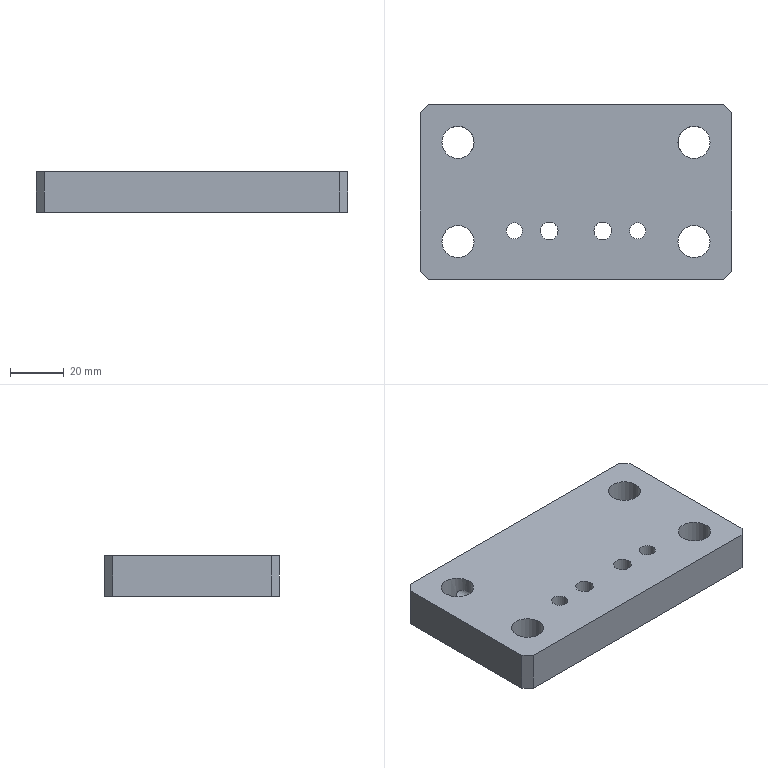Part | NX | features BREP 1 | 1 solid | 29 faces | box 116 x 65 x 15 mm | volume 102539 mm3 | cylinder 14 | plane 12 | cone 3 | commonest cylinder face diameters 5 x4 12 x4 6 x2 6.6 x2 11 x2
STEP:
#1=CARTESIAN_POINT('',(58.,0.,5.));
#2=VERTEX_POINT('',#1);
#3=CARTESIAN_POINT('',(58.,0.,7.5));
#4=DIRECTION('',(1.,0.,0.));
#5=DIRECTION('',(0.,0.,-1.));
#6=AXIS2_PLACEMENT_3D('',#3,#4,#5);
#7=CIRCLE('',#6,2.5);
#8=EDGE_CURVE('',#2,#2,#7,.T.);
#9=ORIENTED_EDGE('',*,*,#8,.F.);
#10=EDGE_LOOP('',(#9));
#11=FACE_BOUND('',#10,.T.);
#12=CARTESIAN_POINT('',(58.,-29.5,15.));
#13=VERTEX_POINT('',#12);
#14=CARTESIAN_POINT('',(58.,29.5,15.));
#15=VERTEX_POINT('',#14);
#16=CARTESIAN_POINT('',(58.,32.5,15.));
#17=DIRECTION('',(0.,1.,0.));
#18=VECTOR('',#17,1000.);
#19=LINE('',#16,#18);
#20=EDGE_CURVE('',#13,#15,#19,.T.);
#21=ORIENTED_EDGE('',*,*,#20,.F.);
#22=CARTESIAN_POINT('',(58.,-29.5,0.));
#23=VERTEX_POINT('',#22);
#24=CARTESIAN_POINT('',(58.,-29.5,15.));
#25=DIRECTION('',(0.,0.,-1.));
#26=VECTOR('',#25,1000.);
#27=LINE('',#24,#26);
#28=EDGE_CURVE('',#13,#23,#27,.T.);
#29=ORIENTED_EDGE('',*,*,#28,.T.);
#30=CARTESIAN_POINT('',(58.,29.5,0.));
#31=VERTEX_POINT('',#30);
#32=CARTESIAN_POINT('',(58.,32.5,0.));
#33=DIRECTION('',(0.,1.,0.));
#34=VECTOR('',#33,1000.);
#35=LINE('',#32,#34);
#36=EDGE_CURVE('',#23,#31,#35,.T.);
#37=ORIENTED_EDGE('',*,*,#36,.T.);
#38=CARTESIAN_POINT('',(58.,29.5,15.));
#39=DIRECTION('',(0.,0.,1.));
#40=VECTOR('',#39,1000.);
#41=LINE('',#38,#40);
#42=EDGE_CURVE('',#31,#15,#41,.T.);
#43=ORIENTED_EDGE('',*,*,#42,.T.);
#44=EDGE_LOOP('',(#21,#29,#37,#43));
#45=FACE_BOUND('',#44,.T.);
#46=CARTESIAN_POINT('',(58.,32.5,15.));
#47=DIRECTION('',(-1.,0.,0.));
#48=DIRECTION('',(0.,0.,-1.));
#49=AXIS2_PLACEMENT_3D('',#46,#47,#48);
#50=PLANE('',#49);
#51=ADVANCED_FACE('',(#11,#45),#50,.F.);
#52=CARTESIAN_POINT('',(37.5,32.5,10.));
#53=VERTEX_POINT('',#52);
#54=CARTESIAN_POINT('',(37.5,32.5,7.5));
#55=DIRECTION('',(0.,1.,0.));
#56=DIRECTION('',(0.,0.,1.));
#57=AXIS2_PLACEMENT_3D('',#54,#55,#56);
#58=CIRCLE('',#57,2.5);
#59=EDGE_CURVE('',#53,#53,#58,.T.);
#60=ORIENTED_EDGE('',*,*,#59,.F.);
#61=EDGE_LOOP('',(#60));
#62=FACE_BOUND('',#61,.T.);
#63=CARTESIAN_POINT('',(-37.5,32.5,10.));
#64=VERTEX_POINT('',#63);
#65=CARTESIAN_POINT('',(-37.5,32.5,7.5));
#66=DIRECTION('',(0.,1.,0.));
#67=DIRECTION('',(0.,0.,1.));
#68=AXIS2_PLACEMENT_3D('',#65,#66,#67);
#69=CIRCLE('',#68,2.5);
#70=EDGE_CURVE('',#64,#64,#69,.T.);
#71=ORIENTED_EDGE('',*,*,#70,.F.);
#72=EDGE_LOOP('',(#71));
#73=FACE_BOUND('',#72,.T.);
#74=CARTESIAN_POINT('',(55.,32.5,15.));
#75=VERTEX_POINT('',#74);
#76=CARTESIAN_POINT('',(-55.,32.5,15.));
#77=VERTEX_POINT('',#76);
#78=CARTESIAN_POINT('',(-58.,32.5,15.));
#79=DIRECTION('',(-1.,0.,0.));
#80=VECTOR('',#79,1000.);
#81=LINE('',#78,#80);
#82=EDGE_CURVE('',#75,#77,#81,.T.);
#83=ORIENTED_EDGE('',*,*,#82,.F.);
#84=CARTESIAN_POINT('',(55.,32.5,0.));
#85=VERTEX_POINT('',#84);
#86=CARTESIAN_POINT('',(55.,32.5,15.));
#87=DIRECTION('',(0.,0.,-1.));
#88=VECTOR('',#87,1000.);
#89=LINE('',#86,#88);
#90=EDGE_CURVE('',#75,#85,#89,.T.);
#91=ORIENTED_EDGE('',*,*,#90,.T.);
#92=CARTESIAN_POINT('',(-55.,32.5,0.));
#93=VERTEX_POINT('',#92);
#94=CARTESIAN_POINT('',(-58.,32.5,0.));
#95=DIRECTION('',(-1.,0.,0.));
#96=VECTOR('',#95,1000.);
#97=LINE('',#94,#96);
#98=EDGE_CURVE('',#85,#93,#97,.T.);
#99=ORIENTED_EDGE('',*,*,#98,.T.);
#100=CARTESIAN_POINT('',(-55.,32.5,15.));
#101=DIRECTION('',(0.,0.,1.));
#102=VECTOR('',#101,1000.);
#103=LINE('',#100,#102);
#104=EDGE_CURVE('',#93,#77,#103,.T.);
#105=ORIENTED_EDGE('',*,*,#104,.T.);
#106=EDGE_LOOP('',(#83,#91,#99,#105));
#107=FACE_BOUND('',#106,.T.);
#108=CARTESIAN_POINT('',(-58.,32.5,15.));
#109=DIRECTION('',(0.,-1.,0.));
#110=DIRECTION('',(0.,0.,1.));
#111=AXIS2_PLACEMENT_3D('',#108,#109,#110);
#112=PLANE('',#111);
#113=ADVANCED_FACE('',(#62,#73,#107),#112,.F.);
#114=CARTESIAN_POINT('',(-58.,29.5,0.));
#115=VERTEX_POINT('',#114);
#116=CARTESIAN_POINT('',(-58.,-29.5,0.));
#117=VERTEX_POINT('',#116);
#118=CARTESIAN_POINT('',(-58.,32.5,0.));
#119=DIRECTION('',(0.,-1.,0.));
#120=VECTOR('',#119,1000.);
#121=LINE('',#118,#120);
#122=EDGE_CURVE('',#115,#117,#121,.T.);
#123=ORIENTED_EDGE('',*,*,#122,.T.);
#124=CARTESIAN_POINT('',(-58.,-29.5,15.));
#125=VERTEX_POINT('',#124);
#126=CARTESIAN_POINT('',(-58.,-29.5,15.));
#127=DIRECTION('',(0.,0.,1.));
#128=VECTOR('',#127,1000.);
#129=LINE('',#126,#128);
#130=EDGE_CURVE('',#117,#125,#129,.T.);
#131=ORIENTED_EDGE('',*,*,#130,.T.);
#132=CARTESIAN_POINT('',(-58.,29.5,15.));
#133=VERTEX_POINT('',#132);
#134=CARTESIAN_POINT('',(-58.,32.5,15.));
#135=DIRECTION('',(0.,-1.,0.));
#136=VECTOR('',#135,1000.);
#137=LINE('',#134,#136);
#138=EDGE_CURVE('',#133,#125,#137,.T.);
#139=ORIENTED_EDGE('',*,*,#138,.F.);
#140=CARTESIAN_POINT('',(-58.,29.5,15.));
#141=DIRECTION('',(0.,0.,-1.));
#142=VECTOR('',#141,1000.);
#143=LINE('',#140,#142);
#144=EDGE_CURVE('',#133,#115,#143,.T.);
#145=ORIENTED_EDGE('',*,*,#144,.T.);
#146=EDGE_LOOP('',(#123,#131,#139,#145));
#147=FACE_BOUND('',#146,.T.);
#148=CARTESIAN_POINT('',(-58.,32.5,15.));
#149=DIRECTION('',(1.,0.,0.));
#150=DIRECTION('',(0.,-1.,0.));
#151=AXIS2_PLACEMENT_3D('',#148,#149,#150);
#152=PLANE('',#151);
#153=ADVANCED_FACE('',(#147),#152,.F.);
#154=CARTESIAN_POINT('',(-55.,-32.5,0.));
#155=VERTEX_POINT('',#154);
#156=CARTESIAN_POINT('',(55.,-32.5,0.));
#157=VERTEX_POINT('',#156);
#158=CARTESIAN_POINT('',(-58.,-32.5,0.));
#159=DIRECTION('',(1.,0.,0.));
#160=VECTOR('',#159,1000.);
#161=LINE('',#158,#160);
#162=EDGE_CURVE('',#155,#157,#161,.T.);
#163=ORIENTED_EDGE('',*,*,#162,.T.);
#164=CARTESIAN_POINT('',(55.,-32.5,15.));
#165=VERTEX_POINT('',#164);
#166=CARTESIAN_POINT('',(55.,-32.5,15.));
#167=DIRECTION('',(0.,0.,1.));
#168=VECTOR('',#167,1000.);
#169=LINE('',#166,#168);
#170=EDGE_CURVE('',#157,#165,#169,.T.);
#171=ORIENTED_EDGE('',*,*,#170,.T.);
#172=CARTESIAN_POINT('',(-55.,-32.5,15.));
#173=VERTEX_POINT('',#172);
#174=CARTESIAN_POINT('',(-58.,-32.5,15.));
#175=DIRECTION('',(1.,0.,0.));
#176=VECTOR('',#175,1000.);
#177=LINE('',#174,#176);
#178=EDGE_CURVE('',#173,#165,#177,.T.);
#179=ORIENTED_EDGE('',*,*,#178,.F.);
#180=CARTESIAN_POINT('',(-55.,-32.5,15.));
#181=DIRECTION('',(0.,0.,-1.));
#182=VECTOR('',#181,1000.);
#183=LINE('',#180,#182);
#184=EDGE_CURVE('',#173,#155,#183,.T.);
#185=ORIENTED_EDGE('',*,*,#184,.T.);
#186=EDGE_LOOP('',(#163,#171,#179,#185));
#187=FACE_BOUND('',#186,.T.);
#188=CARTESIAN_POINT('',(-58.,-32.5,15.));
#189=DIRECTION('',(0.,1.,0.));
#190=DIRECTION('',(0.,0.,-1.));
#191=AXIS2_PLACEMENT_3D('',#188,#189,#190);
#192=PLANE('',#191);
#193=ADVANCED_FACE('',(#187),#192,.F.);
#194=CARTESIAN_POINT('',(-13.3,-14.5,15.));
#195=VERTEX_POINT('',#194);
#196=CARTESIAN_POINT('',(-10.,-14.5,15.));
#197=DIRECTION('',(0.,0.,-1.));
#198=DIRECTION('',(-1.,0.,0.));
#199=AXIS2_PLACEMENT_3D('',#196,#197,#198);
#200=CIRCLE('',#199,3.3);
#201=EDGE_CURVE('',#195,#195,#200,.T.);
#202=ORIENTED_EDGE('',*,*,#201,.T.);
#203=EDGE_LOOP('',(#202));
#204=FACE_BOUND('',#203,.T.);
#205=CARTESIAN_POINT('',(6.7,-14.5,15.));
#206=VERTEX_POINT('',#205);
#207=CARTESIAN_POINT('',(10.,-14.5,15.));
#208=DIRECTION('',(0.,0.,-1.));
#209=DIRECTION('',(-1.,0.,0.));
#210=AXIS2_PLACEMENT_3D('',#207,#208,#209);
#211=CIRCLE('',#210,3.3);
#212=EDGE_CURVE('',#206,#206,#211,.T.);
#213=ORIENTED_EDGE('',*,*,#212,.T.);
#214=EDGE_LOOP('',(#213));
#215=FACE_BOUND('',#214,.T.);
#216=CARTESIAN_POINT('',(26.,-14.5,15.));
#217=VERTEX_POINT('',#216);
#218=CARTESIAN_POINT('',(23.,-14.5,15.));
#219=DIRECTION('',(0.,0.,1.));
#220=DIRECTION('',(1.,0.,0.));
#221=AXIS2_PLACEMENT_3D('',#218,#219,#220);
#222=CIRCLE('',#221,3.);
#223=EDGE_CURVE('',#217,#217,#222,.T.);
#224=ORIENTED_EDGE('',*,*,#223,.F.);
#225=EDGE_LOOP('',(#224));
#226=FACE_BOUND('',#225,.T.);
#227=CARTESIAN_POINT('',(-20.,-14.5,15.));
#228=VERTEX_POINT('',#227);
#229=CARTESIAN_POINT('',(-23.,-14.5,15.));
#230=DIRECTION('',(0.,0.,1.));
#231=DIRECTION('',(1.,0.,0.));
#232=AXIS2_PLACEMENT_3D('',#229,#230,#231);
#233=CIRCLE('',#232,3.);
#234=EDGE_CURVE('',#228,#228,#233,.T.);
#235=ORIENTED_EDGE('',*,*,#234,.F.);
#236=EDGE_LOOP('',(#235));
#237=FACE_BOUND('',#236,.T.);
#238=CARTESIAN_POINT('',(50.,-18.5,15.));
#239=VERTEX_POINT('',#238);
#240=CARTESIAN_POINT('',(44.,-18.5,15.));
#241=DIRECTION('',(0.,0.,1.));
#242=DIRECTION('',(1.,0.,0.));
#243=AXIS2_PLACEMENT_3D('',#240,#241,#242);
#244=CIRCLE('',#243,6.);
#245=EDGE_CURVE('',#239,#239,#244,.T.);
#246=ORIENTED_EDGE('',*,*,#245,.F.);
#247=EDGE_LOOP('',(#246));
#248=FACE_BOUND('',#247,.T.);
#249=CARTESIAN_POINT('',(50.,18.5,15.));
#250=VERTEX_POINT('',#249);
#251=CARTESIAN_POINT('',(44.,18.5,15.));
#252=DIRECTION('',(0.,0.,1.));
#253=DIRECTION('',(1.,0.,0.));
#254=AXIS2_PLACEMENT_3D('',#251,#252,#253);
#255=CIRCLE('',#254,6.);
#256=EDGE_CURVE('',#250,#250,#255,.T.);
#257=ORIENTED_EDGE('',*,*,#256,.F.);
#258=EDGE_LOOP('',(#257));
#259=FACE_BOUND('',#258,.T.);
#260=CARTESIAN_POINT('',(-38.,18.5,15.));
#261=VERTEX_POINT('',#260);
#262=CARTESIAN_POINT('',(-44.,18.5,15.));
#263=DIRECTION('',(0.,0.,1.));
#264=DIRECTION('',(1.,0.,0.));
#265=AXIS2_PLACEMENT_3D('',#262,#263,#264);
#266=CIRCLE('',#265,6.);
#267=EDGE_CURVE('',#261,#261,#266,.T.);
#268=ORIENTED_EDGE('',*,*,#267,.F.);
#269=EDGE_LOOP('',(#268));
#270=FACE_BOUND('',#269,.T.);
#271=CARTESIAN_POINT('',(-38.,-18.5,15.));
#272=VERTEX_POINT('',#271);
#273=CARTESIAN_POINT('',(-44.,-18.5,15.));
#274=DIRECTION('',(0.,0.,1.));
#275=DIRECTION('',(1.,0.,0.));
#276=AXIS2_PLACEMENT_3D('',#273,#274,#275);
#277=CIRCLE('',#276,6.);
#278=EDGE_CURVE('',#272,#272,#277,.T.);
#279=ORIENTED_EDGE('',*,*,#278,.F.);
#280=EDGE_LOOP('',(#279));
#281=FACE_BOUND('',#280,.T.);
#282=ORIENTED_EDGE('',*,*,#178,.T.);
#283=CARTESIAN_POINT('',(43.75,-43.75,15.));
#284=DIRECTION('',(0.7071,0.7071,0.));
#285=VECTOR('',#284,1000.);
#286=LINE('',#283,#285);
#287=EDGE_CURVE('',#165,#13,#286,.T.);
#288=ORIENTED_EDGE('',*,*,#287,.T.);
#289=ORIENTED_EDGE('',*,*,#20,.T.);
#290=CARTESIAN_POINT('',(43.75,43.75,15.));
#291=DIRECTION('',(-0.7071,0.7071,0.));
#292=VECTOR('',#291,1000.);
#293=LINE('',#290,#292);
#294=EDGE_CURVE('',#15,#75,#293,.T.);
#295=ORIENTED_EDGE('',*,*,#294,.T.);
#296=ORIENTED_EDGE('',*,*,#82,.T.);
#297=CARTESIAN_POINT('',(-43.75,43.75,15.));
#298=DIRECTION('',(-0.7071,-0.7071,0.));
#299=VECTOR('',#298,1000.);
#300=LINE('',#297,#299);
#301=EDGE_CURVE('',#77,#133,#300,.T.);
#302=ORIENTED_EDGE('',*,*,#301,.T.);
#303=ORIENTED_EDGE('',*,*,#138,.T.);
#304=CARTESIAN_POINT('',(-43.75,-43.75,15.));
#305=DIRECTION('',(0.7071,-0.7071,0.));
#306=VECTOR('',#305,1000.);
#307=LINE('',#304,#306);
#308=EDGE_CURVE('',#125,#173,#307,.T.);
#309=ORIENTED_EDGE('',*,*,#308,.T.);
#310=EDGE_LOOP('',(#282,#288,#289,#295,#296,#302,#303,#309));
#311=FACE_BOUND('',#310,.T.);
#312=CARTESIAN_POINT('',(0.,0.,15.));
#313=DIRECTION('',(0.,0.,1.));
#314=DIRECTION('',(-1.,0.,0.));
#315=AXIS2_PLACEMENT_3D('',#312,#313,#314);
#316=PLANE('',#315);
#317=ADVANCED_FACE('',(#204,#215,#226,#237,#248,#259,#270,#281,#311),#316,.T.);
#318=CARTESIAN_POINT('',(-15.5,-14.5,0.));
#319=VERTEX_POINT('',#318);
#320=CARTESIAN_POINT('',(-10.,-14.5,0.));
#321=DIRECTION('',(0.,0.,-1.));
#322=DIRECTION('',(-1.,0.,0.));
#323=AXIS2_PLACEMENT_3D('',#320,#321,#322);
#324=CIRCLE('',#323,5.5);
#325=EDGE_CURVE('',#319,#319,#324,.T.);
#326=ORIENTED_EDGE('',*,*,#325,.F.);
#327=EDGE_LOOP('',(#326));
#328=FACE_BOUND('',#327,.T.);
#329=CARTESIAN_POINT('',(4.5,-14.5,0.));
#330=VERTEX_POINT('',#329);
#331=CARTESIAN_POINT('',(10.,-14.5,0.));
#332=DIRECTION('',(0.,0.,-1.));
#333=DIRECTION('',(-1.,0.,0.));
#334=AXIS2_PLACEMENT_3D('',#331,#332,#333);
#335=CIRCLE('',#334,5.5);
#336=EDGE_CURVE('',#330,#330,#335,.T.);
#337=ORIENTED_EDGE('',*,*,#336,.F.);
#338=EDGE_LOOP('',(#337));
#339=FACE_BOUND('',#338,.T.);
#340=CARTESIAN_POINT('',(26.,-14.5,0.));
#341=VERTEX_POINT('',#340);
#342=CARTESIAN_POINT('',(23.,-14.5,0.));
#343=DIRECTION('',(0.,0.,1.));
#344=DIRECTION('',(1.,0.,0.));
#345=AXIS2_PLACEMENT_3D('',#342,#343,#344);
#346=CIRCLE('',#345,3.);
#347=EDGE_CURVE('',#341,#341,#346,.T.);
#348=ORIENTED_EDGE('',*,*,#347,.T.);
#349=EDGE_LOOP('',(#348));
#350=FACE_BOUND('',#349,.T.);
#351=CARTESIAN_POINT('',(-20.,-14.5,0.));
#352=VERTEX_POINT('',#351);
#353=CARTESIAN_POINT('',(-23.,-14.5,0.));
#354=DIRECTION('',(0.,0.,1.));
#355=DIRECTION('',(1.,0.,0.));
#356=AXIS2_PLACEMENT_3D('',#353,#354,#355);
#357=CIRCLE('',#356,3.);
#358=EDGE_CURVE('',#352,#352,#357,.T.);
#359=ORIENTED_EDGE('',*,*,#358,.T.);
#360=EDGE_LOOP('',(#359));
#361=FACE_BOUND('',#360,.T.);
#362=CARTESIAN_POINT('',(50.,-18.5,0.));
#363=VERTEX_POINT('',#362);
#364=CARTESIAN_POINT('',(44.,-18.5,0.));
#365=DIRECTION('',(0.,0.,1.));
#366=DIRECTION('',(1.,0.,0.));
#367=AXIS2_PLACEMENT_3D('',#364,#365,#366);
#368=CIRCLE('',#367,6.);
#369=EDGE_CURVE('',#363,#363,#368,.T.);
#370=ORIENTED_EDGE('',*,*,#369,.T.);
#371=EDGE_LOOP('',(#370));
#372=FACE_BOUND('',#371,.T.);
#373=CARTESIAN_POINT('',(50.,18.5,0.));
#374=VERTEX_POINT('',#373);
#375=CARTESIAN_POINT('',(44.,18.5,0.));
#376=DIRECTION('',(0.,0.,1.));
#377=DIRECTION('',(1.,0.,0.));
#378=AXIS2_PLACEMENT_3D('',#375,#376,#377);
#379=CIRCLE('',#378,6.);
#380=EDGE_CURVE('',#374,#374,#379,.T.);
#381=ORIENTED_EDGE('',*,*,#380,.T.);
#382=EDGE_LOOP('',(#381));
#383=FACE_BOUND('',#382,.T.);
#384=CARTESIAN_POINT('',(-38.,18.5,0.));
#385=VERTEX_POINT('',#384);
#386=CARTESIAN_POINT('',(-44.,18.5,0.));
#387=DIRECTION('',(0.,0.,1.));
#388=DIRECTION('',(1.,0.,0.));
#389=AXIS2_PLACEMENT_3D('',#386,#387,#388);
#390=CIRCLE('',#389,6.);
#391=EDGE_CURVE('',#385,#385,#390,.T.);
#392=ORIENTED_EDGE('',*,*,#391,.T.);
#393=EDGE_LOOP('',(#392));
#394=FACE_BOUND('',#393,.T.);
#395=CARTESIAN_POINT('',(-38.,-18.5,0.));
#396=VERTEX_POINT('',#395);
#397=CARTESIAN_POINT('',(-44.,-18.5,0.));
#398=DIRECTION('',(0.,0.,1.));
#399=DIRECTION('',(1.,0.,0.));
#400=AXIS2_PLACEMENT_3D('',#397,#398,#399);
#401=CIRCLE('',#400,6.);
#402=EDGE_CURVE('',#396,#396,#401,.T.);
#403=ORIENTED_EDGE('',*,*,#402,.T.);
#404=EDGE_LOOP('',(#403));
#405=FACE_BOUND('',#404,.T.);
#406=ORIENTED_EDGE('',*,*,#36,.F.);
#407=CARTESIAN_POINT('',(58.,-29.5,0.));
#408=DIRECTION('',(-0.7071,-0.7071,0.));
#409=VECTOR('',#408,1000.);
#410=LINE('',#407,#409);
#411=EDGE_CURVE('',#23,#157,#410,.T.);
#412=ORIENTED_EDGE('',*,*,#411,.T.);
#413=ORIENTED_EDGE('',*,*,#162,.F.);
#414=CARTESIAN_POINT('',(-55.,-32.5,0.));
#415=DIRECTION('',(-0.7071,0.7071,0.));
#416=VECTOR('',#415,1000.);
#417=LINE('',#414,#416);
#418=EDGE_CURVE('',#155,#117,#417,.T.);
#419=ORIENTED_EDGE('',*,*,#418,.T.);
#420=ORIENTED_EDGE('',*,*,#122,.F.);
#421=CARTESIAN_POINT('',(-58.,29.5,0.));
#422=DIRECTION('',(0.7071,0.7071,0.));
#423=VECTOR('',#422,1000.);
#424=LINE('',#421,#423);
#425=EDGE_CURVE('',#115,#93,#424,.T.);
#426=ORIENTED_EDGE('',*,*,#425,.T.);
#427=ORIENTED_EDGE('',*,*,#98,.F.);
#428=CARTESIAN_POINT('',(55.,32.5,0.));
#429=DIRECTION('',(0.7071,-0.7071,0.));
#430=VECTOR('',#429,1000.);
#431=LINE('',#428,#430);
#432=EDGE_CURVE('',#85,#31,#431,.T.);
#433=ORIENTED_EDGE('',*,*,#432,.T.);
#434=EDGE_LOOP('',(#406,#412,#413,#419,#420,#426,#427,#433));
#435=FACE_BOUND('',#434,.T.);
#436=CARTESIAN_POINT('',(0.,0.,0.));
#437=DIRECTION('',(0.,0.,1.));
#438=DIRECTION('',(-1.,0.,0.));
#439=AXIS2_PLACEMENT_3D('',#436,#437,#438);
#440=PLANE('',#439);
#441=ADVANCED_FACE('',(#328,#339,#350,#361,#372,#383,#394,#405,#435),#440,.F.);
#442=ORIENTED_EDGE('',*,*,#402,.F.);
#443=EDGE_LOOP('',(#442));
#444=FACE_BOUND('',#443,.T.);
#445=ORIENTED_EDGE('',*,*,#278,.T.);
#446=EDGE_LOOP('',(#445));
#447=FACE_BOUND('',#446,.T.);
#448=CARTESIAN_POINT('',(-44.,-18.5,15.));
#449=DIRECTION('',(0.,0.,1.));
#450=DIRECTION('',(-1.,0.,0.));
#451=AXIS2_PLACEMENT_3D('',#448,#449,#450);
#452=CYLINDRICAL_SURFACE('',#451,6.);
#453=ADVANCED_FACE('',(#444,#447),#452,.F.);
#454=CARTESIAN_POINT('',(-38.084,17.5,9.931));
#455=VERTEX_POINT('',#454);
#456=CARTESIAN_POINT('',(-38.084,17.5,5.069));
#457=VERTEX_POINT('',#456);
#458=CARTESIAN_POINT('',(-38.084,17.5,9.931));
#459=CARTESIAN_POINT('',(-38.121,17.28,9.545));
#460=CARTESIAN_POINT('',(-38.219,16.853,8.787));
#461=CARTESIAN_POINT('',(-38.404,16.329,7.497));
#462=CARTESIAN_POINT('',(-38.218,16.855,6.211));
#463=CARTESIAN_POINT('',(-38.121,17.281,5.454));
#464=CARTESIAN_POINT('',(-38.084,17.5,5.069));
#465=B_SPLINE_CURVE_WITH_KNOTS('',3,(#458,#459,#460,#461,#462,#463,#464),.UNSPECIFIED.,.F.,.F.,(4,1,1,1,4),(0.,0.001335,0.002669,0.004004,0.005339),.UNSPECIFIED.);
#466=EDGE_CURVE('',#455,#457,#465,.T.);
#467=ORIENTED_EDGE('',*,*,#466,.T.);
#468=CARTESIAN_POINT('',(-38.084,17.5,5.069));
#469=CARTESIAN_POINT('',(-37.983,18.098,5.045));
#470=CARTESIAN_POINT('',(-37.966,19.305,5.043));
#471=CARTESIAN_POINT('',(-38.461,21.047,5.154));
#472=CARTESIAN_POINT('',(-39.481,22.542,5.725));
#473=CARTESIAN_POINT('',(-40.257,23.185,7.487));
#474=CARTESIAN_POINT('',(-39.492,22.553,9.265));
#475=CARTESIAN_POINT('',(-38.471,21.068,9.843));
#476=CARTESIAN_POINT('',(-37.966,19.32,9.957));
#477=CARTESIAN_POINT('',(-37.983,18.098,9.955));
#478=CARTESIAN_POINT('',(-38.084,17.5,9.931));
#479=B_SPLINE_CURVE_WITH_KNOTS('',3,(#468,#469,#470,#471,#472,#473,#474,#475,#476,#477,#478),.UNSPECIFIED.,.F.,.F.,(4,1,1,1,1,1,1,1,4),(0.,0.001794,0.003588,0.005381,0.007175,0.008969,0.01076,0.01256,0.01435),.UNSPECIFIED.);
#480=EDGE_CURVE('',#457,#455,#479,.T.);
#481=ORIENTED_EDGE('',*,*,#480,.T.);
#482=EDGE_LOOP('',(#467,#481));
#483=FACE_BOUND('',#482,.T.);
#484=ORIENTED_EDGE('',*,*,#391,.F.);
#485=EDGE_LOOP('',(#484));
#486=FACE_BOUND('',#485,.T.);
#487=ORIENTED_EDGE('',*,*,#267,.T.);
#488=EDGE_LOOP('',(#487));
#489=FACE_BOUND('',#488,.T.);
#490=CARTESIAN_POINT('',(-44.,18.5,15.));
#491=DIRECTION('',(0.,0.,1.));
#492=DIRECTION('',(-1.,0.,0.));
#493=AXIS2_PLACEMENT_3D('',#490,#491,#492);
#494=CYLINDRICAL_SURFACE('',#493,6.);
#495=ADVANCED_FACE('',(#483,#486,#489),#494,.F.);
#496=CARTESIAN_POINT('',(38.084,17.5,5.069));
#497=VERTEX_POINT('',#496);
#498=CARTESIAN_POINT('',(38.084,17.5,9.931));
#499=VERTEX_POINT('',#498);
#500=CARTESIAN_POINT('',(38.084,17.5,5.069));
#501=CARTESIAN_POINT('',(38.121,17.28,5.455));
#502=CARTESIAN_POINT('',(38.219,16.853,6.213));
#503=CARTESIAN_POINT('',(38.404,16.329,7.503));
#504=CARTESIAN_POINT('',(38.218,16.855,8.789));
#505=CARTESIAN_POINT('',(38.121,17.281,9.546));
#506=CARTESIAN_POINT('',(38.084,17.5,9.931));
#507=B_SPLINE_CURVE_WITH_KNOTS('',3,(#500,#501,#502,#503,#504,#505,#506),.UNSPECIFIED.,.F.,.F.,(4,1,1,1,4),(0.,0.001335,0.002669,0.004004,0.005339),.UNSPECIFIED.);
#508=EDGE_CURVE('',#497,#499,#507,.T.);
#509=ORIENTED_EDGE('',*,*,#508,.T.);
#510=CARTESIAN_POINT('',(38.084,17.5,9.931));
#511=CARTESIAN_POINT('',(37.983,18.098,9.955));
#512=CARTESIAN_POINT('',(37.966,19.305,9.957));
#513=CARTESIAN_POINT('',(38.461,21.047,9.846));
#514=CARTESIAN_POINT('',(39.481,22.542,9.275));
#515=CARTESIAN_POINT('',(40.257,23.185,7.513));
#516=CARTESIAN_POINT('',(39.492,22.553,5.735));
#517=CARTESIAN_POINT('',(38.471,21.068,5.157));
#518=CARTESIAN_POINT('',(37.966,19.32,5.043));
#519=CARTESIAN_POINT('',(37.983,18.098,5.045));
#520=CARTESIAN_POINT('',(38.084,17.5,5.069));
#521=B_SPLINE_CURVE_WITH_KNOTS('',3,(#510,#511,#512,#513,#514,#515,#516,#517,#518,#519,#520),.UNSPECIFIED.,.F.,.F.,(4,1,1,1,1,1,1,1,4),(0.,0.001794,0.003588,0.005381,0.007175,0.008969,0.01076,0.01256,0.01435),.UNSPECIFIED.);
#522=EDGE_CURVE('',#499,#497,#521,.T.);
#523=ORIENTED_EDGE('',*,*,#522,.T.);
#524=EDGE_LOOP('',(#509,#523));
#525=FACE_BOUND('',#524,.T.);
#526=ORIENTED_EDGE('',*,*,#380,.F.);
#527=EDGE_LOOP('',(#526));
#528=FACE_BOUND('',#527,.T.);
#529=ORIENTED_EDGE('',*,*,#256,.T.);
#530=EDGE_LOOP('',(#529));
#531=FACE_BOUND('',#530,.T.);
#532=CARTESIAN_POINT('',(44.,18.5,15.));
#533=DIRECTION('',(0.,0.,1.));
#534=DIRECTION('',(-1.,0.,0.));
#535=AXIS2_PLACEMENT_3D('',#532,#533,#534);
#536=CYLINDRICAL_SURFACE('',#535,6.);
#537=ADVANCED_FACE('',(#525,#528,#531),#536,.F.);
#538=ORIENTED_EDGE('',*,*,#369,.F.);
#539=EDGE_LOOP('',(#538));
#540=FACE_BOUND('',#539,.T.);
#541=ORIENTED_EDGE('',*,*,#245,.T.);
#542=EDGE_LOOP('',(#541));
#543=FACE_BOUND('',#542,.T.);
#544=CARTESIAN_POINT('',(44.,-18.5,15.));
#545=DIRECTION('',(0.,0.,1.));
#546=DIRECTION('',(-1.,0.,0.));
#547=AXIS2_PLACEMENT_3D('',#544,#545,#546);
#548=CYLINDRICAL_SURFACE('',#547,6.);
#549=ADVANCED_FACE('',(#540,#543),#548,.F.);
#550=ORIENTED_EDGE('',*,*,#287,.F.);
#551=ORIENTED_EDGE('',*,*,#170,.F.);
#552=ORIENTED_EDGE('',*,*,#411,.F.);
#553=ORIENTED_EDGE('',*,*,#28,.F.);
#554=EDGE_LOOP('',(#550,#551,#552,#553));
#555=FACE_BOUND('',#554,.T.);
#556=CARTESIAN_POINT('',(58.,-29.5,15.));
#557=DIRECTION('',(-0.7071,0.7071,0.));
#558=DIRECTION('',(0.,0.,1.));
#559=AXIS2_PLACEMENT_3D('',#556,#557,#558);
#560=PLANE('',#559);
#561=ADVANCED_FACE('',(#555),#560,.F.);
#562=ORIENTED_EDGE('',*,*,#294,.F.);
#563=ORIENTED_EDGE('',*,*,#42,.F.);
#564=ORIENTED_EDGE('',*,*,#432,.F.);
#565=ORIENTED_EDGE('',*,*,#90,.F.);
#566=EDGE_LOOP('',(#562,#563,#564,#565));
#567=FACE_BOUND('',#566,.T.);
#568=CARTESIAN_POINT('',(55.,32.5,15.));
#569=DIRECTION('',(-0.7071,-0.7071,0.));
#570=DIRECTION('',(0.,0.,1.));
#571=AXIS2_PLACEMENT_3D('',#568,#569,#570);
#572=PLANE('',#571);
#573=ADVANCED_FACE('',(#567),#572,.F.);
#574=ORIENTED_EDGE('',*,*,#308,.F.);
#575=ORIENTED_EDGE('',*,*,#130,.F.);
#576=ORIENTED_EDGE('',*,*,#418,.F.);
#577=ORIENTED_EDGE('',*,*,#184,.F.);
#578=EDGE_LOOP('',(#574,#575,#576,#577));
#579=FACE_BOUND('',#578,.T.);
#580=CARTESIAN_POINT('',(-55.,-32.5,15.));
#581=DIRECTION('',(0.7071,0.7071,0.));
#582=DIRECTION('',(0.,0.,1.));
#583=AXIS2_PLACEMENT_3D('',#580,#581,#582);
#584=PLANE('',#583);
#585=ADVANCED_FACE('',(#579),#584,.F.);
#586=ORIENTED_EDGE('',*,*,#301,.F.);
#587=ORIENTED_EDGE('',*,*,#104,.F.);
#588=ORIENTED_EDGE('',*,*,#425,.F.);
#589=ORIENTED_EDGE('',*,*,#144,.F.);
#590=EDGE_LOOP('',(#586,#587,#588,#589));
#591=FACE_BOUND('',#590,.T.);
#592=CARTESIAN_POINT('',(-58.,29.5,15.));
#593=DIRECTION('',(0.7071,-0.7071,0.));
#594=DIRECTION('',(0.,0.,1.));
#595=AXIS2_PLACEMENT_3D('',#592,#593,#594);
#596=PLANE('',#595);
#597=ADVANCED_FACE('',(#591),#596,.F.);
#598=ORIENTED_EDGE('',*,*,#358,.F.);
#599=EDGE_LOOP('',(#598));
#600=FACE_BOUND('',#599,.T.);
#601=ORIENTED_EDGE('',*,*,#234,.T.);
#602=EDGE_LOOP('',(#601));
#603=FACE_BOUND('',#602,.T.);
#604=CARTESIAN_POINT('',(-23.,-14.5,15.));
#605=DIRECTION('',(0.,0.,1.));
#606=DIRECTION('',(-1.,0.,0.));
#607=AXIS2_PLACEMENT_3D('',#604,#605,#606);
#608=CYLINDRICAL_SURFACE('',#607,3.);
#609=ADVANCED_FACE('',(#600,#603),#608,.F.);
#610=ORIENTED_EDGE('',*,*,#347,.F.);
#611=EDGE_LOOP('',(#610));
#612=FACE_BOUND('',#611,.T.);
#613=ORIENTED_EDGE('',*,*,#223,.T.);
#614=EDGE_LOOP('',(#613));
#615=FACE_BOUND('',#614,.T.);
#616=CARTESIAN_POINT('',(23.,-14.5,15.));
#617=DIRECTION('',(0.,0.,1.));
#618=DIRECTION('',(-1.,0.,0.));
#619=AXIS2_PLACEMENT_3D('',#616,#617,#618);
#620=CYLINDRICAL_SURFACE('',#619,3.);
#621=ADVANCED_FACE('',(#612,#615),#620,.F.);
#622=ORIENTED_EDGE('',*,*,#212,.F.);
#623=EDGE_LOOP('',(#622));
#624=FACE_BOUND('',#623,.T.);
#625=CARTESIAN_POINT('',(6.7,-14.5,6.4));
#626=VERTEX_POINT('',#625);
#627=CARTESIAN_POINT('',(10.,-14.5,6.4));
#628=DIRECTION('',(0.,0.,-1.));
#629=DIRECTION('',(-1.,0.,0.));
#630=AXIS2_PLACEMENT_3D('',#627,#628,#629);
#631=CIRCLE('',#630,3.3);
#632=EDGE_CURVE('',#626,#626,#631,.T.);
#633=ORIENTED_EDGE('',*,*,#632,.T.);
#634=EDGE_LOOP('',(#633));
#635=FACE_BOUND('',#634,.T.);
#636=CARTESIAN_POINT('',(10.,-14.5,0.));
#637=DIRECTION('',(0.,0.,-1.));
#638=DIRECTION('',(1.,0.,0.));
#639=AXIS2_PLACEMENT_3D('',#636,#637,#638);
#640=CYLINDRICAL_SURFACE('',#639,3.3);
#641=ADVANCED_FACE('',(#624,#635),#640,.F.);
#642=ORIENTED_EDGE('',*,*,#632,.F.);
#643=EDGE_LOOP('',(#642));
#644=FACE_BOUND('',#643,.T.);
#645=CARTESIAN_POINT('',(4.5,-14.5,6.4));
#646=VERTEX_POINT('',#645);
#647=CARTESIAN_POINT('',(10.,-14.5,6.4));
#648=DIRECTION('',(0.,0.,-1.));
#649=DIRECTION('',(-1.,0.,0.));
#650=AXIS2_PLACEMENT_3D('',#647,#648,#649);
#651=CIRCLE('',#650,5.5);
#652=EDGE_CURVE('',#646,#646,#651,.T.);
#653=ORIENTED_EDGE('',*,*,#652,.T.);
#654=EDGE_LOOP('',(#653));
#655=FACE_BOUND('',#654,.T.);
#656=CARTESIAN_POINT('',(13.3,-14.5,6.4));
#657=DIRECTION('',(0.,0.,1.));
#658=DIRECTION('',(-1.,0.,0.));
#659=AXIS2_PLACEMENT_3D('',#656,#657,#658);
#660=PLANE('',#659);
#661=ADVANCED_FACE('',(#644,#655),#660,.F.);
#662=ORIENTED_EDGE('',*,*,#652,.F.);
#663=EDGE_LOOP('',(#662));
#664=FACE_BOUND('',#663,.T.);
#665=ORIENTED_EDGE('',*,*,#336,.T.);
#666=EDGE_LOOP('',(#665));
#667=FACE_BOUND('',#666,.T.);
#668=CARTESIAN_POINT('',(10.,-14.5,0.));
#669=DIRECTION('',(0.,0.,-1.));
#670=DIRECTION('',(1.,0.,0.));
#671=AXIS2_PLACEMENT_3D('',#668,#669,#670);
#672=CYLINDRICAL_SURFACE('',#671,5.5);
#673=ADVANCED_FACE('',(#664,#667),#672,.F.);
#674=ORIENTED_EDGE('',*,*,#201,.F.);
#675=EDGE_LOOP('',(#674));
#676=FACE_BOUND('',#675,.T.);
#677=CARTESIAN_POINT('',(-13.3,-14.5,6.4));
#678=VERTEX_POINT('',#677);
#679=CARTESIAN_POINT('',(-10.,-14.5,6.4));
#680=DIRECTION('',(0.,0.,-1.));
#681=DIRECTION('',(-1.,0.,0.));
#682=AXIS2_PLACEMENT_3D('',#679,#680,#681);
#683=CIRCLE('',#682,3.3);
#684=EDGE_CURVE('',#678,#678,#683,.T.);
#685=ORIENTED_EDGE('',*,*,#684,.T.);
#686=EDGE_LOOP('',(#685));
#687=FACE_BOUND('',#686,.T.);
#688=CARTESIAN_POINT('',(-10.,-14.5,0.));
#689=DIRECTION('',(0.,0.,-1.));
#690=DIRECTION('',(1.,0.,0.));
#691=AXIS2_PLACEMENT_3D('',#688,#689,#690);
#692=CYLINDRICAL_SURFACE('',#691,3.3);
#693=ADVANCED_FACE('',(#676,#687),#692,.F.);
#694=ORIENTED_EDGE('',*,*,#684,.F.);
#695=EDGE_LOOP('',(#694));
#696=FACE_BOUND('',#695,.T.);
#697=CARTESIAN_POINT('',(-15.5,-14.5,6.4));
#698=VERTEX_POINT('',#697);
#699=CARTESIAN_POINT('',(-10.,-14.5,6.4));
#700=DIRECTION('',(0.,0.,-1.));
#701=DIRECTION('',(-1.,0.,0.));
#702=AXIS2_PLACEMENT_3D('',#699,#700,#701);
#703=CIRCLE('',#702,5.5);
#704=EDGE_CURVE('',#698,#698,#703,.T.);
#705=ORIENTED_EDGE('',*,*,#704,.T.);
#706=EDGE_LOOP('',(#705));
#707=FACE_BOUND('',#706,.T.);
#708=CARTESIAN_POINT('',(-6.7,-14.5,6.4));
#709=DIRECTION('',(0.,0.,1.));
#710=DIRECTION('',(-1.,0.,0.));
#711=AXIS2_PLACEMENT_3D('',#708,#709,#710);
#712=PLANE('',#711);
#713=ADVANCED_FACE('',(#696,#707),#712,.F.);
#714=ORIENTED_EDGE('',*,*,#704,.F.);
#715=EDGE_LOOP('',(#714));
#716=FACE_BOUND('',#715,.T.);
#717=ORIENTED_EDGE('',*,*,#325,.T.);
#718=EDGE_LOOP('',(#717));
#719=FACE_BOUND('',#718,.T.);
#720=CARTESIAN_POINT('',(-10.,-14.5,0.));
#721=DIRECTION('',(0.,0.,-1.));
#722=DIRECTION('',(1.,0.,0.));
#723=AXIS2_PLACEMENT_3D('',#720,#721,#722);
#724=CYLINDRICAL_SURFACE('',#723,5.5);
#725=ADVANCED_FACE('',(#716,#719),#724,.F.);
#726=ORIENTED_EDGE('',*,*,#70,.T.);
#727=EDGE_LOOP('',(#726));
#728=FACE_BOUND('',#727,.T.);
#729=CARTESIAN_POINT('',(-37.5,17.5,7.5));
#730=DIRECTION('',(0.,1.,0.));
#731=DIRECTION('',(0.,0.,1.));
#732=AXIS2_PLACEMENT_3D('',#729,#730,#731);
#733=CIRCLE('',#732,2.5);
#734=EDGE_CURVE('',#455,#457,#733,.T.);
#735=ORIENTED_EDGE('',*,*,#734,.F.);
#736=ORIENTED_EDGE('',*,*,#480,.F.);
#737=EDGE_LOOP('',(#735,#736));
#738=FACE_BOUND('',#737,.T.);
#739=CARTESIAN_POINT('',(-37.5,32.5,7.5));
#740=DIRECTION('',(0.,1.,0.));
#741=DIRECTION('',(0.,0.,-1.));
#742=AXIS2_PLACEMENT_3D('',#739,#740,#741);
#743=CYLINDRICAL_SURFACE('',#742,2.5);
#744=ADVANCED_FACE('',(#728,#738),#743,.F.);
#745=ORIENTED_EDGE('',*,*,#734,.T.);
#746=ORIENTED_EDGE('',*,*,#466,.F.);
#747=EDGE_LOOP('',(#745,#746));
#748=FACE_BOUND('',#747,.T.);
#749=CARTESIAN_POINT('',(-37.5,17.5,7.5));
#750=DIRECTION('',(0.,1.,0.));
#751=DIRECTION('',(0.,0.,-1.));
#752=AXIS2_PLACEMENT_3D('',#749,#750,#751);
#753=CONICAL_SURFACE('',#752,2.5,1.03);
#754=ADVANCED_FACE('',(#748),#753,.F.);
#755=ORIENTED_EDGE('',*,*,#59,.T.);
#756=EDGE_LOOP('',(#755));
#757=FACE_BOUND('',#756,.T.);
#758=CARTESIAN_POINT('',(37.5,17.5,7.5));
#759=DIRECTION('',(0.,1.,0.));
#760=DIRECTION('',(0.,0.,1.));
#761=AXIS2_PLACEMENT_3D('',#758,#759,#760);
#762=CIRCLE('',#761,2.5);
#763=EDGE_CURVE('',#497,#499,#762,.T.);
#764=ORIENTED_EDGE('',*,*,#763,.F.);
#765=ORIENTED_EDGE('',*,*,#522,.F.);
#766=EDGE_LOOP('',(#764,#765));
#767=FACE_BOUND('',#766,.T.);
#768=CARTESIAN_POINT('',(37.5,32.5,7.5));
#769=DIRECTION('',(0.,1.,0.));
#770=DIRECTION('',(0.,0.,-1.));
#771=AXIS2_PLACEMENT_3D('',#768,#769,#770);
#772=CYLINDRICAL_SURFACE('',#771,2.5);
#773=ADVANCED_FACE('',(#757,#767),#772,.F.);
#774=ORIENTED_EDGE('',*,*,#763,.T.);
#775=ORIENTED_EDGE('',*,*,#508,.F.);
#776=EDGE_LOOP('',(#774,#775));
#777=FACE_BOUND('',#776,.T.);
#778=CARTESIAN_POINT('',(37.5,17.5,7.5));
#779=DIRECTION('',(0.,1.,0.));
#780=DIRECTION('',(0.,0.,-1.));
#781=AXIS2_PLACEMENT_3D('',#778,#779,#780);
#782=CONICAL_SURFACE('',#781,2.5,1.03);
#783=ADVANCED_FACE('',(#777),#782,.F.);
#784=CARTESIAN_POINT('',(41.498,0.,7.5));
#785=VERTEX_POINT('',#784);
#786=VERTEX_LOOP('',#785);
#787=FACE_BOUND('',#786,.T.);
#788=CARTESIAN_POINT('',(43.,0.,5.));
#789=VERTEX_POINT('',#788);
#790=CARTESIAN_POINT('',(43.,0.,7.5));
#791=DIRECTION('',(1.,0.,0.));
#792=DIRECTION('',(0.,0.,-1.));
#793=AXIS2_PLACEMENT_3D('',#790,#791,#792);
#794=CIRCLE('',#793,2.5);
#795=EDGE_CURVE('',#789,#789,#794,.T.);
#796=ORIENTED_EDGE('',*,*,#795,.T.);
#797=EDGE_LOOP('',(#796));
#798=FACE_BOUND('',#797,.T.);
#799=CARTESIAN_POINT('',(43.,0.,7.5));
#800=DIRECTION('',(1.,0.,0.));
#801=DIRECTION('',(0.,0.,1.));
#802=AXIS2_PLACEMENT_3D('',#799,#800,#801);
#803=CONICAL_SURFACE('',#802,2.5,1.03);
#804=ADVANCED_FACE('',(#787,#798),#803,.F.);
#805=ORIENTED_EDGE('',*,*,#795,.F.);
#806=EDGE_LOOP('',(#805));
#807=FACE_BOUND('',#806,.T.);
#808=ORIENTED_EDGE('',*,*,#8,.T.);
#809=EDGE_LOOP('',(#808));
#810=FACE_BOUND('',#809,.T.);
#811=CARTESIAN_POINT('',(58.,0.,7.5));
#812=DIRECTION('',(1.,0.,0.));
#813=DIRECTION('',(0.,0.,1.));
#814=AXIS2_PLACEMENT_3D('',#811,#812,#813);
#815=CYLINDRICAL_SURFACE('',#814,2.5);
#816=ADVANCED_FACE('',(#807,#810),#815,.F.);
#817=CLOSED_SHELL('',(#51,#113,#153,#193,#317,#441,#453,#495,#537,#549,#561,#573,#585,#597,#609,#621,#641,#661,#673,#693,#713,#725,#744,#754,#773,#783,#804,#816));
#818=MANIFOLD_SOLID_BREP('',#817);
#819=(LENGTH_UNIT()NAMED_UNIT(*)SI_UNIT(.MILLI.,.METRE.));
#820=UNCERTAINTY_MEASURE_WITH_UNIT(LENGTH_MEASURE(0.0508),#819,'','');
#821=(NAMED_UNIT(*)PLANE_ANGLE_UNIT()SI_UNIT($,.RADIAN.));
#822=(NAMED_UNIT(*)SI_UNIT($,.STERADIAN.)SOLID_ANGLE_UNIT());
#823=(GEOMETRIC_REPRESENTATION_CONTEXT(3)GLOBAL_UNCERTAINTY_ASSIGNED_CONTEXT((#820))GLOBAL_UNIT_ASSIGNED_CONTEXT((#819,#821,#822))REPRESENTATION_CONTEXT('',''));
#824=ADVANCED_BREP_SHAPE_REPRESENTATION('',(#818),#823);